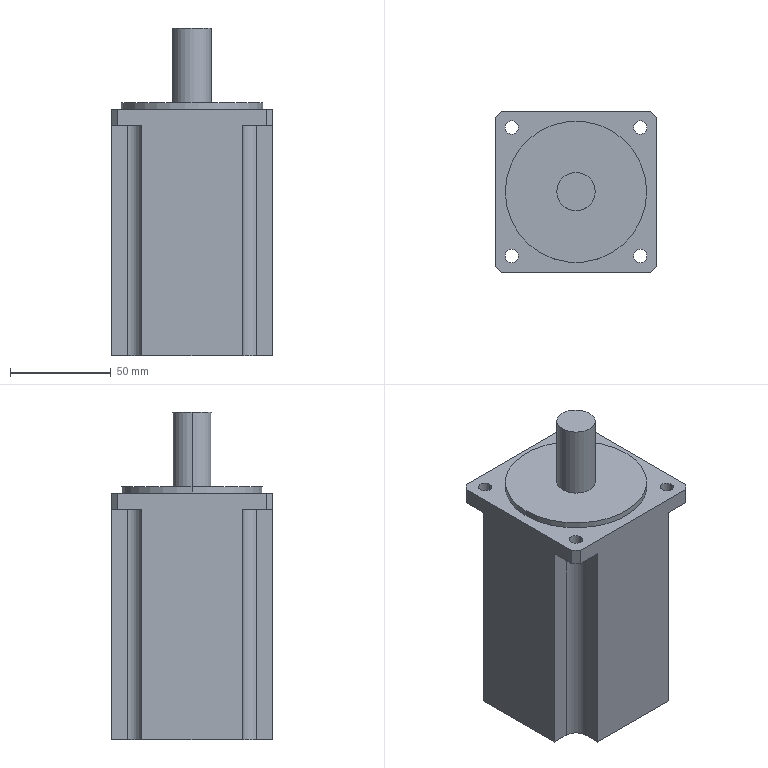Part | Creo | features CURVE 4, DATUM PLANE 3, PROTRUSION 3, CHAMFER 1, COORDINATE SYSTEM 1, CUT 1 | 1 solid | 40 faces | box 80 x 80 x 162.2 mm | volume 703450 mm3 | plane 24 | cylinder 16 | commonest cylinder face diameters 6.6 x8 13.834 x4 19 x2 70 x2
STEP:
#1=CARTESIAN_POINT('',(0.,0.,0.));
#2=DIRECTION('',(0.,0.,1.));
#3=DIRECTION('',(1.,0.,0.));
#4=AXIS2_PLACEMENT_3D('',#1,#2,#3);
#5=CARTESIAN_POINT('',(-24.903,40.,0.));
#6=VERTEX_POINT('',#5);
#7=CARTESIAN_POINT('',(-24.903,31.82,0.));
#8=VERTEX_POINT('',#7);
#9=CARTESIAN_POINT('',(-24.903,40.,0.));
#10=DIRECTION('',(0.,-1.,0.));
#11=VECTOR('',#10,8.18);
#12=LINE('',#9,#11);
#13=EDGE_CURVE('',#6,#8,#12,.T.);
#14=ORIENTED_EDGE('',*,*,#13,.T.);
#15=CARTESIAN_POINT('',(-31.82,24.903,0.));
#16=VERTEX_POINT('',#15);
#17=CARTESIAN_POINT('',(-31.82,31.82,0.));
#18=DIRECTION('',(0.,0.,-1.));
#19=DIRECTION('',(1.,0.,0.));
#20=AXIS2_PLACEMENT_3D('',#17,#18,#19);
#21=CIRCLE('',#20,6.917);
#22=EDGE_CURVE('',#8,#16,#21,.T.);
#23=ORIENTED_EDGE('',*,*,#22,.T.);
#24=CARTESIAN_POINT('',(-40.,24.903,0.));
#25=VERTEX_POINT('',#24);
#26=CARTESIAN_POINT('',(-40.,24.903,0.));
#27=DIRECTION('',(1.,0.,0.));
#28=VECTOR('',#27,8.18);
#29=LINE('',#26,#28);
#30=EDGE_CURVE('',#25,#16,#29,.T.);
#31=ORIENTED_EDGE('',*,*,#30,.F.);
#32=CARTESIAN_POINT('',(-40.,-24.903,0.));
#33=VERTEX_POINT('',#32);
#34=CARTESIAN_POINT('',(-40.,24.903,0.));
#35=DIRECTION('',(0.,-1.,0.));
#36=VECTOR('',#35,49.805);
#37=LINE('',#34,#36);
#38=EDGE_CURVE('',#25,#33,#37,.T.);
#39=ORIENTED_EDGE('',*,*,#38,.T.);
#40=CARTESIAN_POINT('',(-31.82,-24.903,0.));
#41=VERTEX_POINT('',#40);
#42=CARTESIAN_POINT('',(-40.,-24.903,0.));
#43=DIRECTION('',(1.,0.,0.));
#44=VECTOR('',#43,8.18);
#45=LINE('',#42,#44);
#46=EDGE_CURVE('',#33,#41,#45,.T.);
#47=ORIENTED_EDGE('',*,*,#46,.T.);
#48=CARTESIAN_POINT('',(-24.903,-31.82,0.));
#49=VERTEX_POINT('',#48);
#50=CARTESIAN_POINT('',(-31.82,-31.82,0.));
#51=DIRECTION('',(0.,0.,-1.));
#52=DIRECTION('',(0.,1.,0.));
#53=AXIS2_PLACEMENT_3D('',#50,#51,#52);
#54=CIRCLE('',#53,6.917);
#55=EDGE_CURVE('',#41,#49,#54,.T.);
#56=ORIENTED_EDGE('',*,*,#55,.T.);
#57=CARTESIAN_POINT('',(-24.903,-40.,0.));
#58=VERTEX_POINT('',#57);
#59=CARTESIAN_POINT('',(-24.903,-40.,0.));
#60=DIRECTION('',(0.,1.,0.));
#61=VECTOR('',#60,8.18);
#62=LINE('',#59,#61);
#63=EDGE_CURVE('',#58,#49,#62,.T.);
#64=ORIENTED_EDGE('',*,*,#63,.F.);
#65=CARTESIAN_POINT('',(24.903,-40.,0.));
#66=VERTEX_POINT('',#65);
#67=CARTESIAN_POINT('',(-24.903,-40.,0.));
#68=DIRECTION('',(1.,0.,0.));
#69=VECTOR('',#68,49.805);
#70=LINE('',#67,#69);
#71=EDGE_CURVE('',#58,#66,#70,.T.);
#72=ORIENTED_EDGE('',*,*,#71,.T.);
#73=CARTESIAN_POINT('',(24.903,-31.82,0.));
#74=VERTEX_POINT('',#73);
#75=CARTESIAN_POINT('',(24.903,-40.,0.));
#76=DIRECTION('',(0.,1.,0.));
#77=VECTOR('',#76,8.18);
#78=LINE('',#75,#77);
#79=EDGE_CURVE('',#66,#74,#78,.T.);
#80=ORIENTED_EDGE('',*,*,#79,.T.);
#81=CARTESIAN_POINT('',(31.82,-24.903,0.));
#82=VERTEX_POINT('',#81);
#83=CARTESIAN_POINT('',(31.82,-31.82,0.));
#84=DIRECTION('',(0.,0.,-1.));
#85=DIRECTION('',(-1.,0.,0.));
#86=AXIS2_PLACEMENT_3D('',#83,#84,#85);
#87=CIRCLE('',#86,6.917);
#88=EDGE_CURVE('',#74,#82,#87,.T.);
#89=ORIENTED_EDGE('',*,*,#88,.T.);
#90=CARTESIAN_POINT('',(40.,-24.903,0.));
#91=VERTEX_POINT('',#90);
#92=CARTESIAN_POINT('',(40.,-24.903,0.));
#93=DIRECTION('',(-1.,0.,0.));
#94=VECTOR('',#93,8.18);
#95=LINE('',#92,#94);
#96=EDGE_CURVE('',#91,#82,#95,.T.);
#97=ORIENTED_EDGE('',*,*,#96,.F.);
#98=CARTESIAN_POINT('',(40.,24.903,0.));
#99=VERTEX_POINT('',#98);
#100=CARTESIAN_POINT('',(40.,-24.903,0.));
#101=DIRECTION('',(0.,1.,0.));
#102=VECTOR('',#101,49.805);
#103=LINE('',#100,#102);
#104=EDGE_CURVE('',#91,#99,#103,.T.);
#105=ORIENTED_EDGE('',*,*,#104,.T.);
#106=CARTESIAN_POINT('',(31.82,24.903,0.));
#107=VERTEX_POINT('',#106);
#108=CARTESIAN_POINT('',(40.,24.903,0.));
#109=DIRECTION('',(-1.,0.,0.));
#110=VECTOR('',#109,8.18);
#111=LINE('',#108,#110);
#112=EDGE_CURVE('',#99,#107,#111,.T.);
#113=ORIENTED_EDGE('',*,*,#112,.T.);
#114=CARTESIAN_POINT('',(24.903,31.82,0.));
#115=VERTEX_POINT('',#114);
#116=CARTESIAN_POINT('',(31.82,31.82,0.));
#117=DIRECTION('',(0.,0.,-1.));
#118=DIRECTION('',(0.,-1.,0.));
#119=AXIS2_PLACEMENT_3D('',#116,#117,#118);
#120=CIRCLE('',#119,6.917);
#121=EDGE_CURVE('',#107,#115,#120,.T.);
#122=ORIENTED_EDGE('',*,*,#121,.T.);
#123=CARTESIAN_POINT('',(24.903,40.,0.));
#124=VERTEX_POINT('',#123);
#125=CARTESIAN_POINT('',(24.903,40.,0.));
#126=DIRECTION('',(0.,-1.,0.));
#127=VECTOR('',#126,8.18);
#128=LINE('',#125,#127);
#129=EDGE_CURVE('',#124,#115,#128,.T.);
#130=ORIENTED_EDGE('',*,*,#129,.F.);
#131=CARTESIAN_POINT('',(24.903,40.,0.));
#132=DIRECTION('',(-1.,0.,0.));
#133=VECTOR('',#132,49.805);
#134=LINE('',#131,#133);
#135=EDGE_CURVE('',#124,#6,#134,.T.);
#136=ORIENTED_EDGE('',*,*,#135,.T.);
#137=EDGE_LOOP('',(#14,#23,#31,#39,#47,#56,#64,#72,#80,#89,#97,#105,#113,#122,#130,#136));
#138=FACE_OUTER_BOUND('',#137,.F.);
#139=CARTESIAN_POINT('',(0.,0.,0.));
#140=DIRECTION('',(0.,0.,1.));
#141=DIRECTION('',(1.,0.,0.));
#142=AXIS2_PLACEMENT_3D('',#139,#140,#141);
#143=PLANE('',#142);
#144=ADVANCED_FACE('',(#138),#143,.F.);
#145=ORIENTED_EDGE('',*,*,#13,.F.);
#146=CARTESIAN_POINT('',(-24.903,40.,114.2));
#147=VERTEX_POINT('',#146);
#148=CARTESIAN_POINT('',(-24.903,40.,0.));
#149=DIRECTION('',(0.,0.,1.));
#150=VECTOR('',#149,114.2);
#151=LINE('',#148,#150);
#152=EDGE_CURVE('',#6,#147,#151,.T.);
#153=ORIENTED_EDGE('',*,*,#152,.T.);
#154=CARTESIAN_POINT('',(-24.903,31.82,114.2));
#155=VERTEX_POINT('',#154);
#156=CARTESIAN_POINT('',(-24.903,40.,114.2));
#157=DIRECTION('',(0.,-1.,0.));
#158=VECTOR('',#157,8.18);
#159=LINE('',#156,#158);
#160=EDGE_CURVE('',#147,#155,#159,.T.);
#161=ORIENTED_EDGE('',*,*,#160,.T.);
#162=CARTESIAN_POINT('',(-24.903,31.82,0.));
#163=DIRECTION('',(0.,0.,1.));
#164=VECTOR('',#163,114.2);
#165=LINE('',#162,#164);
#166=EDGE_CURVE('',#8,#155,#165,.T.);
#167=ORIENTED_EDGE('',*,*,#166,.F.);
#168=EDGE_LOOP('',(#145,#153,#161,#167));
#169=FACE_OUTER_BOUND('',#168,.F.);
#170=CARTESIAN_POINT('',(-24.903,40.,0.));
#171=DIRECTION('',(1.,0.,0.));
#172=DIRECTION('',(0.,-1.,0.));
#173=AXIS2_PLACEMENT_3D('',#170,#171,#172);
#174=PLANE('',#173);
#175=ADVANCED_FACE('',(#169),#174,.F.);
#176=CARTESIAN_POINT('',(-37.,40.,122.2));
#177=VERTEX_POINT('',#176);
#178=CARTESIAN_POINT('',(-37.,40.,114.2));
#179=VERTEX_POINT('',#178);
#180=CARTESIAN_POINT('',(-37.,40.,122.2));
#181=DIRECTION('',(0.,0.,-1.));
#182=VECTOR('',#181,8.);
#183=LINE('',#180,#182);
#184=EDGE_CURVE('',#177,#179,#183,.T.);
#185=ORIENTED_EDGE('',*,*,#184,.T.);
#186=CARTESIAN_POINT('',(-24.903,40.,114.2));
#187=DIRECTION('',(-1.,0.,0.));
#188=VECTOR('',#187,12.097);
#189=LINE('',#186,#188);
#190=EDGE_CURVE('',#147,#179,#189,.T.);
#191=ORIENTED_EDGE('',*,*,#190,.F.);
#192=ORIENTED_EDGE('',*,*,#152,.F.);
#193=ORIENTED_EDGE('',*,*,#135,.F.);
#194=CARTESIAN_POINT('',(24.903,40.,114.2));
#195=VERTEX_POINT('',#194);
#196=CARTESIAN_POINT('',(24.903,40.,0.));
#197=DIRECTION('',(0.,0.,1.));
#198=VECTOR('',#197,114.2);
#199=LINE('',#196,#198);
#200=EDGE_CURVE('',#124,#195,#199,.T.);
#201=ORIENTED_EDGE('',*,*,#200,.T.);
#202=CARTESIAN_POINT('',(37.,40.,114.2));
#203=VERTEX_POINT('',#202);
#204=CARTESIAN_POINT('',(37.,40.,114.2));
#205=DIRECTION('',(-1.,0.,0.));
#206=VECTOR('',#205,12.097);
#207=LINE('',#204,#206);
#208=EDGE_CURVE('',#203,#195,#207,.T.);
#209=ORIENTED_EDGE('',*,*,#208,.F.);
#210=CARTESIAN_POINT('',(37.,40.,122.2));
#211=VERTEX_POINT('',#210);
#212=CARTESIAN_POINT('',(37.,40.,122.2));
#213=DIRECTION('',(0.,0.,-1.));
#214=VECTOR('',#213,8.);
#215=LINE('',#212,#214);
#216=EDGE_CURVE('',#211,#203,#215,.T.);
#217=ORIENTED_EDGE('',*,*,#216,.F.);
#218=CARTESIAN_POINT('',(37.,40.,122.2));
#219=DIRECTION('',(-1.,0.,0.));
#220=VECTOR('',#219,74.);
#221=LINE('',#218,#220);
#222=EDGE_CURVE('',#211,#177,#221,.T.);
#223=ORIENTED_EDGE('',*,*,#222,.T.);
#224=EDGE_LOOP('',(#185,#191,#192,#193,#201,#209,#217,#223));
#225=FACE_OUTER_BOUND('',#224,.F.);
#226=CARTESIAN_POINT('',(40.,40.,0.));
#227=DIRECTION('',(0.,1.,0.));
#228=DIRECTION('',(-1.,0.,0.));
#229=AXIS2_PLACEMENT_3D('',#226,#227,#228);
#230=PLANE('',#229);
#231=ADVANCED_FACE('',(#225),#230,.T.);
#232=CARTESIAN_POINT('',(-40.,37.,114.2));
#233=VERTEX_POINT('',#232);
#234=CARTESIAN_POINT('',(-40.,37.,114.2));
#235=DIRECTION('',(0.7071,0.7071,0.));
#236=VECTOR('',#235,4.243);
#237=LINE('',#234,#236);
#238=EDGE_CURVE('',#233,#179,#237,.T.);
#239=ORIENTED_EDGE('',*,*,#238,.T.);
#240=ORIENTED_EDGE('',*,*,#184,.F.);
#241=CARTESIAN_POINT('',(-40.,37.,122.2));
#242=VERTEX_POINT('',#241);
#243=CARTESIAN_POINT('',(-37.,40.,122.2));
#244=DIRECTION('',(-0.7071,-0.7071,0.));
#245=VECTOR('',#244,4.243);
#246=LINE('',#243,#245);
#247=EDGE_CURVE('',#177,#242,#246,.T.);
#248=ORIENTED_EDGE('',*,*,#247,.T.);
#249=CARTESIAN_POINT('',(-40.,37.,122.2));
#250=DIRECTION('',(0.,0.,-1.));
#251=VECTOR('',#250,8.);
#252=LINE('',#249,#251);
#253=EDGE_CURVE('',#242,#233,#252,.T.);
#254=ORIENTED_EDGE('',*,*,#253,.T.);
#255=EDGE_LOOP('',(#239,#240,#248,#254));
#256=FACE_OUTER_BOUND('',#255,.F.);
#257=CARTESIAN_POINT('',(-38.5,38.5,118.2));
#258=DIRECTION('',(-0.7071,0.7071,0.));
#259=DIRECTION('',(0.7071,0.7071,0.));
#260=AXIS2_PLACEMENT_3D('',#257,#258,#259);
#261=PLANE('',#260);
#262=ADVANCED_FACE('',(#256),#261,.T.);
#263=ORIENTED_EDGE('',*,*,#238,.F.);
#264=CARTESIAN_POINT('',(-40.,24.903,114.2));
#265=VERTEX_POINT('',#264);
#266=CARTESIAN_POINT('',(-40.,37.,114.2));
#267=DIRECTION('',(0.,-1.,0.));
#268=VECTOR('',#267,12.097);
#269=LINE('',#266,#268);
#270=EDGE_CURVE('',#233,#265,#269,.T.);
#271=ORIENTED_EDGE('',*,*,#270,.T.);
#272=CARTESIAN_POINT('',(-31.82,24.903,114.2));
#273=VERTEX_POINT('',#272);
#274=CARTESIAN_POINT('',(-31.82,24.903,114.2));
#275=DIRECTION('',(-1.,0.,0.));
#276=VECTOR('',#275,8.18);
#277=LINE('',#274,#276);
#278=EDGE_CURVE('',#273,#265,#277,.T.);
#279=ORIENTED_EDGE('',*,*,#278,.F.);
#280=CARTESIAN_POINT('',(-31.82,31.82,114.2));
#281=DIRECTION('',(0.,0.,-1.));
#282=DIRECTION('',(1.,0.,0.));
#283=AXIS2_PLACEMENT_3D('',#280,#281,#282);
#284=CIRCLE('',#283,6.917);
#285=EDGE_CURVE('',#155,#273,#284,.T.);
#286=ORIENTED_EDGE('',*,*,#285,.F.);
#287=ORIENTED_EDGE('',*,*,#160,.F.);
#288=ORIENTED_EDGE('',*,*,#190,.T.);
#289=EDGE_LOOP('',(#263,#271,#279,#286,#287,#288));
#290=FACE_OUTER_BOUND('',#289,.F.);
#291=CARTESIAN_POINT('',(-35.12,31.82,114.2));
#292=VERTEX_POINT('',#291);
#293=CARTESIAN_POINT('',(-28.52,31.82,114.2));
#294=VERTEX_POINT('',#293);
#295=CARTESIAN_POINT('',(-31.82,31.82,114.2));
#296=DIRECTION('',(0.,0.,1.));
#297=DIRECTION('',(-1.,0.,0.));
#298=AXIS2_PLACEMENT_3D('',#295,#296,#297);
#299=CIRCLE('',#298,3.3);
#300=EDGE_CURVE('',#292,#294,#299,.T.);
#301=ORIENTED_EDGE('',*,*,#300,.F.);
#302=CARTESIAN_POINT('',(-31.82,31.82,114.2));
#303=DIRECTION('',(0.,0.,1.));
#304=DIRECTION('',(1.,0.,0.));
#305=AXIS2_PLACEMENT_3D('',#302,#303,#304);
#306=CIRCLE('',#305,3.3);
#307=EDGE_CURVE('',#294,#292,#306,.T.);
#308=ORIENTED_EDGE('',*,*,#307,.F.);
#309=EDGE_LOOP('',(#301,#308));
#310=FACE_BOUND('',#309,.F.);
#311=CARTESIAN_POINT('',(0.,0.,114.2));
#312=DIRECTION('',(0.,0.,-1.));
#313=DIRECTION('',(-1.,0.,0.));
#314=AXIS2_PLACEMENT_3D('',#311,#312,#313);
#315=PLANE('',#314);
#316=ADVANCED_FACE('',(#290,#310),#315,.T.);
#317=CARTESIAN_POINT('',(-37.,-40.,114.2));
#318=VERTEX_POINT('',#317);
#319=CARTESIAN_POINT('',(-40.,-37.,114.2));
#320=VERTEX_POINT('',#319);
#321=CARTESIAN_POINT('',(-37.,-40.,114.2));
#322=DIRECTION('',(-0.7071,0.7071,0.));
#323=VECTOR('',#322,4.243);
#324=LINE('',#321,#323);
#325=EDGE_CURVE('',#318,#320,#324,.T.);
#326=ORIENTED_EDGE('',*,*,#325,.F.);
#327=CARTESIAN_POINT('',(-24.903,-40.,114.2));
#328=VERTEX_POINT('',#327);
#329=CARTESIAN_POINT('',(-37.,-40.,114.2));
#330=DIRECTION('',(1.,0.,0.));
#331=VECTOR('',#330,12.097);
#332=LINE('',#329,#331);
#333=EDGE_CURVE('',#318,#328,#332,.T.);
#334=ORIENTED_EDGE('',*,*,#333,.T.);
#335=CARTESIAN_POINT('',(-24.903,-31.82,114.2));
#336=VERTEX_POINT('',#335);
#337=CARTESIAN_POINT('',(-24.903,-31.82,114.2));
#338=DIRECTION('',(0.,-1.,0.));
#339=VECTOR('',#338,8.18);
#340=LINE('',#337,#339);
#341=EDGE_CURVE('',#336,#328,#340,.T.);
#342=ORIENTED_EDGE('',*,*,#341,.F.);
#343=CARTESIAN_POINT('',(-31.82,-24.903,114.2));
#344=VERTEX_POINT('',#343);
#345=CARTESIAN_POINT('',(-31.82,-31.82,114.2));
#346=DIRECTION('',(0.,0.,-1.));
#347=DIRECTION('',(0.,1.,0.));
#348=AXIS2_PLACEMENT_3D('',#345,#346,#347);
#349=CIRCLE('',#348,6.917);
#350=EDGE_CURVE('',#344,#336,#349,.T.);
#351=ORIENTED_EDGE('',*,*,#350,.F.);
#352=CARTESIAN_POINT('',(-40.,-24.903,114.2));
#353=VERTEX_POINT('',#352);
#354=CARTESIAN_POINT('',(-40.,-24.903,114.2));
#355=DIRECTION('',(1.,0.,0.));
#356=VECTOR('',#355,8.18);
#357=LINE('',#354,#356);
#358=EDGE_CURVE('',#353,#344,#357,.T.);
#359=ORIENTED_EDGE('',*,*,#358,.F.);
#360=CARTESIAN_POINT('',(-40.,-24.903,114.2));
#361=DIRECTION('',(0.,-1.,0.));
#362=VECTOR('',#361,12.097);
#363=LINE('',#360,#362);
#364=EDGE_CURVE('',#353,#320,#363,.T.);
#365=ORIENTED_EDGE('',*,*,#364,.T.);
#366=EDGE_LOOP('',(#326,#334,#342,#351,#359,#365));
#367=FACE_OUTER_BOUND('',#366,.F.);
#368=CARTESIAN_POINT('',(-35.12,-31.82,114.2));
#369=VERTEX_POINT('',#368);
#370=CARTESIAN_POINT('',(-28.52,-31.82,114.2));
#371=VERTEX_POINT('',#370);
#372=CARTESIAN_POINT('',(-31.82,-31.82,114.2));
#373=DIRECTION('',(0.,0.,1.));
#374=DIRECTION('',(-1.,0.,0.));
#375=AXIS2_PLACEMENT_3D('',#372,#373,#374);
#376=CIRCLE('',#375,3.3);
#377=EDGE_CURVE('',#369,#371,#376,.T.);
#378=ORIENTED_EDGE('',*,*,#377,.F.);
#379=CARTESIAN_POINT('',(-31.82,-31.82,114.2));
#380=DIRECTION('',(0.,0.,1.));
#381=DIRECTION('',(1.,0.,0.));
#382=AXIS2_PLACEMENT_3D('',#379,#380,#381);
#383=CIRCLE('',#382,3.3);
#384=EDGE_CURVE('',#371,#369,#383,.T.);
#385=ORIENTED_EDGE('',*,*,#384,.F.);
#386=EDGE_LOOP('',(#378,#385));
#387=FACE_BOUND('',#386,.F.);
#388=CARTESIAN_POINT('',(0.,0.,114.2));
#389=DIRECTION('',(0.,0.,-1.));
#390=DIRECTION('',(-1.,0.,0.));
#391=AXIS2_PLACEMENT_3D('',#388,#389,#390);
#392=PLANE('',#391);
#393=ADVANCED_FACE('',(#367,#387),#392,.T.);
#394=CARTESIAN_POINT('',(40.,-37.,114.2));
#395=VERTEX_POINT('',#394);
#396=CARTESIAN_POINT('',(37.,-40.,114.2));
#397=VERTEX_POINT('',#396);
#398=CARTESIAN_POINT('',(40.,-37.,114.2));
#399=DIRECTION('',(-0.7071,-0.7071,0.));
#400=VECTOR('',#399,4.243);
#401=LINE('',#398,#400);
#402=EDGE_CURVE('',#395,#397,#401,.T.);
#403=ORIENTED_EDGE('',*,*,#402,.F.);
#404=CARTESIAN_POINT('',(40.,-24.903,114.2));
#405=VERTEX_POINT('',#404);
#406=CARTESIAN_POINT('',(40.,-37.,114.2));
#407=DIRECTION('',(0.,1.,0.));
#408=VECTOR('',#407,12.097);
#409=LINE('',#406,#408);
#410=EDGE_CURVE('',#395,#405,#409,.T.);
#411=ORIENTED_EDGE('',*,*,#410,.T.);
#412=CARTESIAN_POINT('',(31.82,-24.903,114.2));
#413=VERTEX_POINT('',#412);
#414=CARTESIAN_POINT('',(31.82,-24.903,114.2));
#415=DIRECTION('',(1.,0.,0.));
#416=VECTOR('',#415,8.18);
#417=LINE('',#414,#416);
#418=EDGE_CURVE('',#413,#405,#417,.T.);
#419=ORIENTED_EDGE('',*,*,#418,.F.);
#420=CARTESIAN_POINT('',(24.903,-31.82,114.2));
#421=VERTEX_POINT('',#420);
#422=CARTESIAN_POINT('',(31.82,-31.82,114.2));
#423=DIRECTION('',(0.,0.,-1.));
#424=DIRECTION('',(-1.,0.,0.));
#425=AXIS2_PLACEMENT_3D('',#422,#423,#424);
#426=CIRCLE('',#425,6.917);
#427=EDGE_CURVE('',#421,#413,#426,.T.);
#428=ORIENTED_EDGE('',*,*,#427,.F.);
#429=CARTESIAN_POINT('',(24.903,-40.,114.2));
#430=VERTEX_POINT('',#429);
#431=CARTESIAN_POINT('',(24.903,-40.,114.2));
#432=DIRECTION('',(0.,1.,0.));
#433=VECTOR('',#432,8.18);
#434=LINE('',#431,#433);
#435=EDGE_CURVE('',#430,#421,#434,.T.);
#436=ORIENTED_EDGE('',*,*,#435,.F.);
#437=CARTESIAN_POINT('',(24.903,-40.,114.2));
#438=DIRECTION('',(1.,0.,0.));
#439=VECTOR('',#438,12.097);
#440=LINE('',#437,#439);
#441=EDGE_CURVE('',#430,#397,#440,.T.);
#442=ORIENTED_EDGE('',*,*,#441,.T.);
#443=EDGE_LOOP('',(#403,#411,#419,#428,#436,#442));
#444=FACE_OUTER_BOUND('',#443,.F.);
#445=CARTESIAN_POINT('',(28.52,-31.82,114.2));
#446=VERTEX_POINT('',#445);
#447=CARTESIAN_POINT('',(35.12,-31.82,114.2));
#448=VERTEX_POINT('',#447);
#449=CARTESIAN_POINT('',(31.82,-31.82,114.2));
#450=DIRECTION('',(0.,0.,1.));
#451=DIRECTION('',(-1.,0.,0.));
#452=AXIS2_PLACEMENT_3D('',#449,#450,#451);
#453=CIRCLE('',#452,3.3);
#454=EDGE_CURVE('',#446,#448,#453,.T.);
#455=ORIENTED_EDGE('',*,*,#454,.F.);
#456=CARTESIAN_POINT('',(31.82,-31.82,114.2));
#457=DIRECTION('',(0.,0.,1.));
#458=DIRECTION('',(1.,0.,0.));
#459=AXIS2_PLACEMENT_3D('',#456,#457,#458);
#460=CIRCLE('',#459,3.3);
#461=EDGE_CURVE('',#448,#446,#460,.T.);
#462=ORIENTED_EDGE('',*,*,#461,.F.);
#463=EDGE_LOOP('',(#455,#462));
#464=FACE_BOUND('',#463,.F.);
#465=CARTESIAN_POINT('',(0.,0.,114.2));
#466=DIRECTION('',(0.,0.,-1.));
#467=DIRECTION('',(-1.,0.,0.));
#468=AXIS2_PLACEMENT_3D('',#465,#466,#467);
#469=PLANE('',#468);
#470=ADVANCED_FACE('',(#444,#464),#469,.T.);
#471=CARTESIAN_POINT('',(40.,37.,114.2));
#472=VERTEX_POINT('',#471);
#473=CARTESIAN_POINT('',(37.,40.,114.2));
#474=DIRECTION('',(0.7071,-0.7071,0.));
#475=VECTOR('',#474,4.243);
#476=LINE('',#473,#475);
#477=EDGE_CURVE('',#203,#472,#476,.T.);
#478=ORIENTED_EDGE('',*,*,#477,.F.);
#479=ORIENTED_EDGE('',*,*,#208,.T.);
#480=CARTESIAN_POINT('',(24.903,31.82,114.2));
#481=VERTEX_POINT('',#480);
#482=CARTESIAN_POINT('',(24.903,31.82,114.2));
#483=DIRECTION('',(0.,1.,0.));
#484=VECTOR('',#483,8.18);
#485=LINE('',#482,#484);
#486=EDGE_CURVE('',#481,#195,#485,.T.);
#487=ORIENTED_EDGE('',*,*,#486,.F.);
#488=CARTESIAN_POINT('',(31.82,24.903,114.2));
#489=VERTEX_POINT('',#488);
#490=CARTESIAN_POINT('',(31.82,31.82,114.2));
#491=DIRECTION('',(0.,0.,-1.));
#492=DIRECTION('',(0.,-1.,0.));
#493=AXIS2_PLACEMENT_3D('',#490,#491,#492);
#494=CIRCLE('',#493,6.917);
#495=EDGE_CURVE('',#489,#481,#494,.T.);
#496=ORIENTED_EDGE('',*,*,#495,.F.);
#497=CARTESIAN_POINT('',(40.,24.903,114.2));
#498=VERTEX_POINT('',#497);
#499=CARTESIAN_POINT('',(40.,24.903,114.2));
#500=DIRECTION('',(-1.,0.,0.));
#501=VECTOR('',#500,8.18);
#502=LINE('',#499,#501);
#503=EDGE_CURVE('',#498,#489,#502,.T.);
#504=ORIENTED_EDGE('',*,*,#503,.F.);
#505=CARTESIAN_POINT('',(40.,24.903,114.2));
#506=DIRECTION('',(0.,1.,0.));
#507=VECTOR('',#506,12.097);
#508=LINE('',#505,#507);
#509=EDGE_CURVE('',#498,#472,#508,.T.);
#510=ORIENTED_EDGE('',*,*,#509,.T.);
#511=EDGE_LOOP('',(#478,#479,#487,#496,#504,#510));
#512=FACE_OUTER_BOUND('',#511,.F.);
#513=CARTESIAN_POINT('',(28.52,31.82,114.2));
#514=VERTEX_POINT('',#513);
#515=CARTESIAN_POINT('',(35.12,31.82,114.2));
#516=VERTEX_POINT('',#515);
#517=CARTESIAN_POINT('',(31.82,31.82,114.2));
#518=DIRECTION('',(0.,0.,1.));
#519=DIRECTION('',(-1.,0.,0.));
#520=AXIS2_PLACEMENT_3D('',#517,#518,#519);
#521=CIRCLE('',#520,3.3);
#522=EDGE_CURVE('',#514,#516,#521,.T.);
#523=ORIENTED_EDGE('',*,*,#522,.F.);
#524=CARTESIAN_POINT('',(31.82,31.82,114.2));
#525=DIRECTION('',(0.,0.,1.));
#526=DIRECTION('',(1.,0.,0.));
#527=AXIS2_PLACEMENT_3D('',#524,#525,#526);
#528=CIRCLE('',#527,3.3);
#529=EDGE_CURVE('',#516,#514,#528,.T.);
#530=ORIENTED_EDGE('',*,*,#529,.F.);
#531=EDGE_LOOP('',(#523,#530));
#532=FACE_BOUND('',#531,.F.);
#533=CARTESIAN_POINT('',(0.,0.,114.2));
#534=DIRECTION('',(0.,0.,-1.));
#535=DIRECTION('',(-1.,0.,0.));
#536=AXIS2_PLACEMENT_3D('',#533,#534,#535);
#537=PLANE('',#536);
#538=ADVANCED_FACE('',(#512,#532),#537,.T.);
#539=ORIENTED_EDGE('',*,*,#454,.T.);
#540=CARTESIAN_POINT('',(35.12,-31.82,122.2));
#541=VERTEX_POINT('',#540);
#542=CARTESIAN_POINT('',(35.12,-31.82,114.2));
#543=DIRECTION('',(0.,0.,1.));
#544=VECTOR('',#543,8.);
#545=LINE('',#542,#544);
#546=EDGE_CURVE('',#448,#541,#545,.T.);
#547=ORIENTED_EDGE('',*,*,#546,.T.);
#548=CARTESIAN_POINT('',(28.52,-31.82,122.2));
#549=VERTEX_POINT('',#548);
#550=CARTESIAN_POINT('',(31.82,-31.82,122.2));
#551=DIRECTION('',(0.,0.,-1.));
#552=DIRECTION('',(1.,0.,0.));
#553=AXIS2_PLACEMENT_3D('',#550,#551,#552);
#554=CIRCLE('',#553,3.3);
#555=EDGE_CURVE('',#541,#549,#554,.T.);
#556=ORIENTED_EDGE('',*,*,#555,.T.);
#557=CARTESIAN_POINT('',(28.52,-31.82,114.2));
#558=DIRECTION('',(0.,0.,1.));
#559=VECTOR('',#558,8.);
#560=LINE('',#557,#559);
#561=EDGE_CURVE('',#446,#549,#560,.T.);
#562=ORIENTED_EDGE('',*,*,#561,.F.);
#563=EDGE_LOOP('',(#539,#547,#556,#562));
#564=FACE_OUTER_BOUND('',#563,.F.);
#565=CARTESIAN_POINT('',(31.82,-31.82,0.));
#566=DIRECTION('',(0.,0.,1.));
#567=DIRECTION('',(1.,0.,0.));
#568=AXIS2_PLACEMENT_3D('',#565,#566,#567);
#569=CYLINDRICAL_SURFACE('',#568,3.3);
#570=ADVANCED_FACE('',(#564),#569,.F.);
#571=ORIENTED_EDGE('',*,*,#461,.T.);
#572=ORIENTED_EDGE('',*,*,#561,.T.);
#573=CARTESIAN_POINT('',(31.82,-31.82,122.2));
#574=DIRECTION('',(0.,0.,-1.));
#575=DIRECTION('',(-1.,0.,0.));
#576=AXIS2_PLACEMENT_3D('',#573,#574,#575);
#577=CIRCLE('',#576,3.3);
#578=EDGE_CURVE('',#549,#541,#577,.T.);
#579=ORIENTED_EDGE('',*,*,#578,.T.);
#580=ORIENTED_EDGE('',*,*,#546,.F.);
#581=EDGE_LOOP('',(#571,#572,#579,#580));
#582=FACE_OUTER_BOUND('',#581,.F.);
#583=CARTESIAN_POINT('',(31.82,-31.82,0.));
#584=DIRECTION('',(0.,0.,1.));
#585=DIRECTION('',(1.,0.,0.));
#586=AXIS2_PLACEMENT_3D('',#583,#584,#585);
#587=CYLINDRICAL_SURFACE('',#586,3.3);
#588=ADVANCED_FACE('',(#582),#587,.F.);
#589=ORIENTED_EDGE('',*,*,#247,.F.);
#590=ORIENTED_EDGE('',*,*,#222,.F.);
#591=CARTESIAN_POINT('',(40.,37.,122.2));
#592=VERTEX_POINT('',#591);
#593=CARTESIAN_POINT('',(40.,37.,122.2));
#594=DIRECTION('',(-0.7071,0.7071,0.));
#595=VECTOR('',#594,4.243);
#596=LINE('',#593,#595);
#597=EDGE_CURVE('',#592,#211,#596,.T.);
#598=ORIENTED_EDGE('',*,*,#597,.F.);
#599=CARTESIAN_POINT('',(40.,-37.,122.2));
#600=VERTEX_POINT('',#599);
#601=CARTESIAN_POINT('',(40.,-37.,122.2));
#602=DIRECTION('',(0.,1.,0.));
#603=VECTOR('',#602,74.);
#604=LINE('',#601,#603);
#605=EDGE_CURVE('',#600,#592,#604,.T.);
#606=ORIENTED_EDGE('',*,*,#605,.F.);
#607=CARTESIAN_POINT('',(37.,-40.,122.2));
#608=VERTEX_POINT('',#607);
#609=CARTESIAN_POINT('',(37.,-40.,122.2));
#610=DIRECTION('',(0.7071,0.7071,0.));
#611=VECTOR('',#610,4.243);
#612=LINE('',#609,#611);
#613=EDGE_CURVE('',#608,#600,#612,.T.);
#614=ORIENTED_EDGE('',*,*,#613,.F.);
#615=CARTESIAN_POINT('',(-37.,-40.,122.2));
#616=VERTEX_POINT('',#615);
#617=CARTESIAN_POINT('',(-37.,-40.,122.2));
#618=DIRECTION('',(1.,0.,0.));
#619=VECTOR('',#618,74.);
#620=LINE('',#617,#619);
#621=EDGE_CURVE('',#616,#608,#620,.T.);
#622=ORIENTED_EDGE('',*,*,#621,.F.);
#623=CARTESIAN_POINT('',(-40.,-37.,122.2));
#624=VERTEX_POINT('',#623);
#625=CARTESIAN_POINT('',(-40.,-37.,122.2));
#626=DIRECTION('',(0.7071,-0.7071,0.));
#627=VECTOR('',#626,4.243);
#628=LINE('',#625,#627);
#629=EDGE_CURVE('',#624,#616,#628,.T.);
#630=ORIENTED_EDGE('',*,*,#629,.F.);
#631=CARTESIAN_POINT('',(-40.,37.,122.2));
#632=DIRECTION('',(0.,-1.,0.));
#633=VECTOR('',#632,74.);
#634=LINE('',#631,#633);
#635=EDGE_CURVE('',#242,#624,#634,.T.);
#636=ORIENTED_EDGE('',*,*,#635,.F.);
#637=EDGE_LOOP('',(#589,#590,#598,#606,#614,#622,#630,#636));
#638=FACE_OUTER_BOUND('',#637,.F.);
#639=CARTESIAN_POINT('',(-28.52,31.82,122.2));
#640=VERTEX_POINT('',#639);
#641=CARTESIAN_POINT('',(-35.12,31.82,122.2));
#642=VERTEX_POINT('',#641);
#643=CARTESIAN_POINT('',(-31.82,31.82,122.2));
#644=DIRECTION('',(0.,0.,-1.));
#645=DIRECTION('',(1.,0.,0.));
#646=AXIS2_PLACEMENT_3D('',#643,#644,#645);
#647=CIRCLE('',#646,3.3);
#648=EDGE_CURVE('',#640,#642,#647,.T.);
#649=ORIENTED_EDGE('',*,*,#648,.F.);
#650=CARTESIAN_POINT('',(-31.82,31.82,122.2));
#651=DIRECTION('',(0.,0.,-1.));
#652=DIRECTION('',(-1.,0.,0.));
#653=AXIS2_PLACEMENT_3D('',#650,#651,#652);
#654=CIRCLE('',#653,3.3);
#655=EDGE_CURVE('',#642,#640,#654,.T.);
#656=ORIENTED_EDGE('',*,*,#655,.F.);
#657=EDGE_LOOP('',(#649,#656));
#658=FACE_BOUND('',#657,.F.);
#659=CARTESIAN_POINT('',(-28.52,-31.82,122.2));
#660=VERTEX_POINT('',#659);
#661=CARTESIAN_POINT('',(-35.12,-31.82,122.2));
#662=VERTEX_POINT('',#661);
#663=CARTESIAN_POINT('',(-31.82,-31.82,122.2));
#664=DIRECTION('',(0.,0.,-1.));
#665=DIRECTION('',(1.,0.,0.));
#666=AXIS2_PLACEMENT_3D('',#663,#664,#665);
#667=CIRCLE('',#666,3.3);
#668=EDGE_CURVE('',#660,#662,#667,.T.);
#669=ORIENTED_EDGE('',*,*,#668,.F.);
#670=CARTESIAN_POINT('',(-31.82,-31.82,122.2));
#671=DIRECTION('',(0.,0.,-1.));
#672=DIRECTION('',(-1.,0.,0.));
#673=AXIS2_PLACEMENT_3D('',#670,#671,#672);
#674=CIRCLE('',#673,3.3);
#675=EDGE_CURVE('',#662,#660,#674,.T.);
#676=ORIENTED_EDGE('',*,*,#675,.F.);
#677=EDGE_LOOP('',(#669,#676));
#678=FACE_BOUND('',#677,.F.);
#679=ORIENTED_EDGE('',*,*,#555,.F.);
#680=ORIENTED_EDGE('',*,*,#578,.F.);
#681=EDGE_LOOP('',(#679,#680));
#682=FACE_BOUND('',#681,.F.);
#683=CARTESIAN_POINT('',(35.,0.,122.2));
#684=VERTEX_POINT('',#683);
#685=CARTESIAN_POINT('',(-35.,0.,122.2));
#686=VERTEX_POINT('',#685);
#687=CARTESIAN_POINT('',(0.,0.,122.2));
#688=DIRECTION('',(0.,0.,1.));
#689=DIRECTION('',(1.,0.,0.));
#690=AXIS2_PLACEMENT_3D('',#687,#688,#689);
#691=CIRCLE('',#690,35.);
#692=EDGE_CURVE('',#684,#686,#691,.T.);
#693=ORIENTED_EDGE('',*,*,#692,.T.);
#694=CARTESIAN_POINT('',(0.,0.,122.2));
#695=DIRECTION('',(0.,0.,1.));
#696=DIRECTION('',(-1.,0.,0.));
#697=AXIS2_PLACEMENT_3D('',#694,#695,#696);
#698=CIRCLE('',#697,35.);
#699=EDGE_CURVE('',#686,#684,#698,.T.);
#700=ORIENTED_EDGE('',*,*,#699,.T.);
#701=EDGE_LOOP('',(#693,#700));
#702=FACE_BOUND('',#701,.F.);
#703=CARTESIAN_POINT('',(35.12,31.82,122.2));
#704=VERTEX_POINT('',#703);
#705=CARTESIAN_POINT('',(28.52,31.82,122.2));
#706=VERTEX_POINT('',#705);
#707=CARTESIAN_POINT('',(31.82,31.82,122.2));
#708=DIRECTION('',(0.,0.,-1.));
#709=DIRECTION('',(1.,0.,0.));
#710=AXIS2_PLACEMENT_3D('',#707,#708,#709);
#711=CIRCLE('',#710,3.3);
#712=EDGE_CURVE('',#704,#706,#711,.T.);
#713=ORIENTED_EDGE('',*,*,#712,.F.);
#714=CARTESIAN_POINT('',(31.82,31.82,122.2));
#715=DIRECTION('',(0.,0.,-1.));
#716=DIRECTION('',(-1.,0.,0.));
#717=AXIS2_PLACEMENT_3D('',#714,#715,#716);
#718=CIRCLE('',#717,3.3);
#719=EDGE_CURVE('',#706,#704,#718,.T.);
#720=ORIENTED_EDGE('',*,*,#719,.F.);
#721=EDGE_LOOP('',(#713,#720));
#722=FACE_BOUND('',#721,.F.);
#723=CARTESIAN_POINT('',(0.,0.,122.2));
#724=DIRECTION('',(0.,0.,1.));
#725=DIRECTION('',(1.,0.,0.));
#726=AXIS2_PLACEMENT_3D('',#723,#724,#725);
#727=PLANE('',#726);
#728=ADVANCED_FACE('',(#638,#658,#678,#682,#702,#722),#727,.T.);
#729=ORIENTED_EDGE('',*,*,#522,.T.);
#730=CARTESIAN_POINT('',(35.12,31.82,114.2));
#731=DIRECTION('',(0.,0.,1.));
#732=VECTOR('',#731,8.);
#733=LINE('',#730,#732);
#734=EDGE_CURVE('',#516,#704,#733,.T.);
#735=ORIENTED_EDGE('',*,*,#734,.T.);
#736=ORIENTED_EDGE('',*,*,#712,.T.);
#737=CARTESIAN_POINT('',(28.52,31.82,114.2));
#738=DIRECTION('',(0.,0.,1.));
#739=VECTOR('',#738,8.);
#740=LINE('',#737,#739);
#741=EDGE_CURVE('',#514,#706,#740,.T.);
#742=ORIENTED_EDGE('',*,*,#741,.F.);
#743=EDGE_LOOP('',(#729,#735,#736,#742));
#744=FACE_OUTER_BOUND('',#743,.F.);
#745=CARTESIAN_POINT('',(31.82,31.82,0.));
#746=DIRECTION('',(0.,0.,1.));
#747=DIRECTION('',(1.,0.,0.));
#748=AXIS2_PLACEMENT_3D('',#745,#746,#747);
#749=CYLINDRICAL_SURFACE('',#748,3.3);
#750=ADVANCED_FACE('',(#744),#749,.F.);
#751=ORIENTED_EDGE('',*,*,#529,.T.);
#752=ORIENTED_EDGE('',*,*,#741,.T.);
#753=ORIENTED_EDGE('',*,*,#719,.T.);
#754=ORIENTED_EDGE('',*,*,#734,.F.);
#755=EDGE_LOOP('',(#751,#752,#753,#754));
#756=FACE_OUTER_BOUND('',#755,.F.);
#757=CARTESIAN_POINT('',(31.82,31.82,0.));
#758=DIRECTION('',(0.,0.,1.));
#759=DIRECTION('',(1.,0.,0.));
#760=AXIS2_PLACEMENT_3D('',#757,#758,#759);
#761=CYLINDRICAL_SURFACE('',#760,3.3);
#762=ADVANCED_FACE('',(#756),#761,.F.);
#763=ORIENTED_EDGE('',*,*,#300,.T.);
#764=CARTESIAN_POINT('',(-28.52,31.82,114.2));
#765=DIRECTION('',(0.,0.,1.));
#766=VECTOR('',#765,8.);
#767=LINE('',#764,#766);
#768=EDGE_CURVE('',#294,#640,#767,.T.);
#769=ORIENTED_EDGE('',*,*,#768,.T.);
#770=ORIENTED_EDGE('',*,*,#648,.T.);
#771=CARTESIAN_POINT('',(-35.12,31.82,114.2));
#772=DIRECTION('',(0.,0.,1.));
#773=VECTOR('',#772,8.);
#774=LINE('',#771,#773);
#775=EDGE_CURVE('',#292,#642,#774,.T.);
#776=ORIENTED_EDGE('',*,*,#775,.F.);
#777=EDGE_LOOP('',(#763,#769,#770,#776));
#778=FACE_OUTER_BOUND('',#777,.F.);
#779=CARTESIAN_POINT('',(-31.82,31.82,0.));
#780=DIRECTION('',(0.,0.,1.));
#781=DIRECTION('',(1.,0.,0.));
#782=AXIS2_PLACEMENT_3D('',#779,#780,#781);
#783=CYLINDRICAL_SURFACE('',#782,3.3);
#784=ADVANCED_FACE('',(#778),#783,.F.);
#785=ORIENTED_EDGE('',*,*,#307,.T.);
#786=ORIENTED_EDGE('',*,*,#775,.T.);
#787=ORIENTED_EDGE('',*,*,#655,.T.);
#788=ORIENTED_EDGE('',*,*,#768,.F.);
#789=EDGE_LOOP('',(#785,#786,#787,#788));
#790=FACE_OUTER_BOUND('',#789,.F.);
#791=CARTESIAN_POINT('',(-31.82,31.82,0.));
#792=DIRECTION('',(0.,0.,1.));
#793=DIRECTION('',(1.,0.,0.));
#794=AXIS2_PLACEMENT_3D('',#791,#792,#793);
#795=CYLINDRICAL_SURFACE('',#794,3.3);
#796=ADVANCED_FACE('',(#790),#795,.F.);
#797=ORIENTED_EDGE('',*,*,#377,.T.);
#798=CARTESIAN_POINT('',(-28.52,-31.82,114.2));
#799=DIRECTION('',(0.,0.,1.));
#800=VECTOR('',#799,8.);
#801=LINE('',#798,#800);
#802=EDGE_CURVE('',#371,#660,#801,.T.);
#803=ORIENTED_EDGE('',*,*,#802,.T.);
#804=ORIENTED_EDGE('',*,*,#668,.T.);
#805=CARTESIAN_POINT('',(-35.12,-31.82,114.2));
#806=DIRECTION('',(0.,0.,1.));
#807=VECTOR('',#806,8.);
#808=LINE('',#805,#807);
#809=EDGE_CURVE('',#369,#662,#808,.T.);
#810=ORIENTED_EDGE('',*,*,#809,.F.);
#811=EDGE_LOOP('',(#797,#803,#804,#810));
#812=FACE_OUTER_BOUND('',#811,.F.);
#813=CARTESIAN_POINT('',(-31.82,-31.82,0.));
#814=DIRECTION('',(0.,0.,1.));
#815=DIRECTION('',(1.,0.,0.));
#816=AXIS2_PLACEMENT_3D('',#813,#814,#815);
#817=CYLINDRICAL_SURFACE('',#816,3.3);
#818=ADVANCED_FACE('',(#812),#817,.F.);
#819=ORIENTED_EDGE('',*,*,#384,.T.);
#820=ORIENTED_EDGE('',*,*,#809,.T.);
#821=ORIENTED_EDGE('',*,*,#675,.T.);
#822=ORIENTED_EDGE('',*,*,#802,.F.);
#823=EDGE_LOOP('',(#819,#820,#821,#822));
#824=FACE_OUTER_BOUND('',#823,.F.);
#825=CARTESIAN_POINT('',(-31.82,-31.82,0.));
#826=DIRECTION('',(0.,0.,1.));
#827=DIRECTION('',(1.,0.,0.));
#828=AXIS2_PLACEMENT_3D('',#825,#826,#827);
#829=CYLINDRICAL_SURFACE('',#828,3.3);
#830=ADVANCED_FACE('',(#824),#829,.F.);
#831=ORIENTED_EDGE('',*,*,#692,.F.);
#832=CARTESIAN_POINT('',(35.,0.,125.2));
#833=VERTEX_POINT('',#832);
#834=CARTESIAN_POINT('',(35.,0.,122.2));
#835=DIRECTION('',(0.,0.,1.));
#836=VECTOR('',#835,3.);
#837=LINE('',#834,#836);
#838=EDGE_CURVE('',#684,#833,#837,.T.);
#839=ORIENTED_EDGE('',*,*,#838,.T.);
#840=CARTESIAN_POINT('',(-35.,0.,125.2));
#841=VERTEX_POINT('',#840);
#842=CARTESIAN_POINT('',(0.,0.,125.2));
#843=DIRECTION('',(0.,0.,1.));
#844=DIRECTION('',(1.,0.,0.));
#845=AXIS2_PLACEMENT_3D('',#842,#843,#844);
#846=CIRCLE('',#845,35.);
#847=EDGE_CURVE('',#833,#841,#846,.T.);
#848=ORIENTED_EDGE('',*,*,#847,.T.);
#849=CARTESIAN_POINT('',(-35.,0.,122.2));
#850=DIRECTION('',(0.,0.,1.));
#851=VECTOR('',#850,3.);
#852=LINE('',#849,#851);
#853=EDGE_CURVE('',#686,#841,#852,.T.);
#854=ORIENTED_EDGE('',*,*,#853,.F.);
#855=EDGE_LOOP('',(#831,#839,#848,#854));
#856=FACE_OUTER_BOUND('',#855,.F.);
#857=CARTESIAN_POINT('',(0.,0.,122.2));
#858=DIRECTION('',(0.,0.,1.));
#859=DIRECTION('',(1.,0.,0.));
#860=AXIS2_PLACEMENT_3D('',#857,#858,#859);
#861=CYLINDRICAL_SURFACE('',#860,35.);
#862=ADVANCED_FACE('',(#856),#861,.T.);
#863=ORIENTED_EDGE('',*,*,#699,.F.);
#864=ORIENTED_EDGE('',*,*,#853,.T.);
#865=CARTESIAN_POINT('',(0.,0.,125.2));
#866=DIRECTION('',(0.,0.,1.));
#867=DIRECTION('',(-1.,0.,0.));
#868=AXIS2_PLACEMENT_3D('',#865,#866,#867);
#869=CIRCLE('',#868,35.);
#870=EDGE_CURVE('',#841,#833,#869,.T.);
#871=ORIENTED_EDGE('',*,*,#870,.T.);
#872=ORIENTED_EDGE('',*,*,#838,.F.);
#873=EDGE_LOOP('',(#863,#864,#871,#872));
#874=FACE_OUTER_BOUND('',#873,.F.);
#875=CARTESIAN_POINT('',(0.,0.,122.2));
#876=DIRECTION('',(0.,0.,1.));
#877=DIRECTION('',(1.,0.,0.));
#878=AXIS2_PLACEMENT_3D('',#875,#876,#877);
#879=CYLINDRICAL_SURFACE('',#878,35.);
#880=ADVANCED_FACE('',(#874),#879,.T.);
#881=ORIENTED_EDGE('',*,*,#847,.F.);
#882=ORIENTED_EDGE('',*,*,#870,.F.);
#883=EDGE_LOOP('',(#881,#882));
#884=FACE_OUTER_BOUND('',#883,.F.);
#885=CARTESIAN_POINT('',(9.5,0.,125.2));
#886=VERTEX_POINT('',#885);
#887=CARTESIAN_POINT('',(-9.5,0.,125.2));
#888=VERTEX_POINT('',#887);
#889=CARTESIAN_POINT('',(0.,0.,125.2));
#890=DIRECTION('',(0.,0.,1.));
#891=DIRECTION('',(1.,0.,0.));
#892=AXIS2_PLACEMENT_3D('',#889,#890,#891);
#893=CIRCLE('',#892,9.5);
#894=EDGE_CURVE('',#886,#888,#893,.T.);
#895=ORIENTED_EDGE('',*,*,#894,.T.);
#896=CARTESIAN_POINT('',(0.,0.,125.2));
#897=DIRECTION('',(0.,0.,1.));
#898=DIRECTION('',(-1.,0.,0.));
#899=AXIS2_PLACEMENT_3D('',#896,#897,#898);
#900=CIRCLE('',#899,9.5);
#901=EDGE_CURVE('',#888,#886,#900,.T.);
#902=ORIENTED_EDGE('',*,*,#901,.T.);
#903=EDGE_LOOP('',(#895,#902));
#904=FACE_BOUND('',#903,.F.);
#905=CARTESIAN_POINT('',(0.,0.,125.2));
#906=DIRECTION('',(0.,0.,1.));
#907=DIRECTION('',(1.,0.,0.));
#908=AXIS2_PLACEMENT_3D('',#905,#906,#907);
#909=PLANE('',#908);
#910=ADVANCED_FACE('',(#884,#904),#909,.T.);
#911=ORIENTED_EDGE('',*,*,#894,.F.);
#912=CARTESIAN_POINT('',(9.5,0.,162.2));
#913=VERTEX_POINT('',#912);
#914=CARTESIAN_POINT('',(9.5,0.,125.2));
#915=DIRECTION('',(0.,0.,1.));
#916=VECTOR('',#915,37.);
#917=LINE('',#914,#916);
#918=EDGE_CURVE('',#886,#913,#917,.T.);
#919=ORIENTED_EDGE('',*,*,#918,.T.);
#920=CARTESIAN_POINT('',(-9.5,0.,162.2));
#921=VERTEX_POINT('',#920);
#922=CARTESIAN_POINT('',(0.,0.,162.2));
#923=DIRECTION('',(0.,0.,1.));
#924=DIRECTION('',(1.,0.,0.));
#925=AXIS2_PLACEMENT_3D('',#922,#923,#924);
#926=CIRCLE('',#925,9.5);
#927=EDGE_CURVE('',#913,#921,#926,.T.);
#928=ORIENTED_EDGE('',*,*,#927,.T.);
#929=CARTESIAN_POINT('',(-9.5,0.,125.2));
#930=DIRECTION('',(0.,0.,1.));
#931=VECTOR('',#930,37.);
#932=LINE('',#929,#931);
#933=EDGE_CURVE('',#888,#921,#932,.T.);
#934=ORIENTED_EDGE('',*,*,#933,.F.);
#935=EDGE_LOOP('',(#911,#919,#928,#934));
#936=FACE_OUTER_BOUND('',#935,.F.);
#937=CARTESIAN_POINT('',(0.,0.,125.2));
#938=DIRECTION('',(0.,0.,1.));
#939=DIRECTION('',(1.,0.,0.));
#940=AXIS2_PLACEMENT_3D('',#937,#938,#939);
#941=CYLINDRICAL_SURFACE('',#940,9.5);
#942=ADVANCED_FACE('',(#936),#941,.T.);
#943=ORIENTED_EDGE('',*,*,#901,.F.);
#944=ORIENTED_EDGE('',*,*,#933,.T.);
#945=CARTESIAN_POINT('',(0.,0.,162.2));
#946=DIRECTION('',(0.,0.,1.));
#947=DIRECTION('',(-1.,0.,0.));
#948=AXIS2_PLACEMENT_3D('',#945,#946,#947);
#949=CIRCLE('',#948,9.5);
#950=EDGE_CURVE('',#921,#913,#949,.T.);
#951=ORIENTED_EDGE('',*,*,#950,.T.);
#952=ORIENTED_EDGE('',*,*,#918,.F.);
#953=EDGE_LOOP('',(#943,#944,#951,#952));
#954=FACE_OUTER_BOUND('',#953,.F.);
#955=CARTESIAN_POINT('',(0.,0.,125.2));
#956=DIRECTION('',(0.,0.,1.));
#957=DIRECTION('',(1.,0.,0.));
#958=AXIS2_PLACEMENT_3D('',#955,#956,#957);
#959=CYLINDRICAL_SURFACE('',#958,9.5);
#960=ADVANCED_FACE('',(#954),#959,.T.);
#961=ORIENTED_EDGE('',*,*,#927,.F.);
#962=ORIENTED_EDGE('',*,*,#950,.F.);
#963=EDGE_LOOP('',(#961,#962));
#964=FACE_OUTER_BOUND('',#963,.F.);
#965=CARTESIAN_POINT('',(0.,0.,162.2));
#966=DIRECTION('',(0.,0.,1.));
#967=DIRECTION('',(1.,0.,0.));
#968=AXIS2_PLACEMENT_3D('',#965,#966,#967);
#969=PLANE('',#968);
#970=ADVANCED_FACE('',(#964),#969,.T.);
#971=ORIENTED_EDGE('',*,*,#477,.T.);
#972=CARTESIAN_POINT('',(40.,37.,122.2));
#973=DIRECTION('',(0.,0.,-1.));
#974=VECTOR('',#973,8.);
#975=LINE('',#972,#974);
#976=EDGE_CURVE('',#592,#472,#975,.T.);
#977=ORIENTED_EDGE('',*,*,#976,.F.);
#978=ORIENTED_EDGE('',*,*,#597,.T.);
#979=ORIENTED_EDGE('',*,*,#216,.T.);
#980=EDGE_LOOP('',(#971,#977,#978,#979));
#981=FACE_OUTER_BOUND('',#980,.F.);
#982=CARTESIAN_POINT('',(38.5,38.5,118.2));
#983=DIRECTION('',(0.7071,0.7071,0.));
#984=DIRECTION('',(0.7071,-0.7071,0.));
#985=AXIS2_PLACEMENT_3D('',#982,#983,#984);
#986=PLANE('',#985);
#987=ADVANCED_FACE('',(#981),#986,.T.);
#988=CARTESIAN_POINT('',(40.,-37.,122.2));
#989=DIRECTION('',(0.,0.,-1.));
#990=VECTOR('',#989,8.);
#991=LINE('',#988,#990);
#992=EDGE_CURVE('',#600,#395,#991,.T.);
#993=ORIENTED_EDGE('',*,*,#992,.F.);
#994=ORIENTED_EDGE('',*,*,#605,.T.);
#995=ORIENTED_EDGE('',*,*,#976,.T.);
#996=ORIENTED_EDGE('',*,*,#509,.F.);
#997=CARTESIAN_POINT('',(40.,24.903,0.));
#998=DIRECTION('',(0.,0.,1.));
#999=VECTOR('',#998,114.2);
#1000=LINE('',#997,#999);
#1001=EDGE_CURVE('',#99,#498,#1000,.T.);
#1002=ORIENTED_EDGE('',*,*,#1001,.F.);
#1003=ORIENTED_EDGE('',*,*,#104,.F.);
#1004=CARTESIAN_POINT('',(40.,-24.903,0.));
#1005=DIRECTION('',(0.,0.,1.));
#1006=VECTOR('',#1005,114.2);
#1007=LINE('',#1004,#1006);
#1008=EDGE_CURVE('',#91,#405,#1007,.T.);
#1009=ORIENTED_EDGE('',*,*,#1008,.T.);
#1010=ORIENTED_EDGE('',*,*,#410,.F.);
#1011=EDGE_LOOP('',(#993,#994,#995,#996,#1002,#1003,#1009,#1010));
#1012=FACE_OUTER_BOUND('',#1011,.F.);
#1013=CARTESIAN_POINT('',(40.,-40.,0.));
#1014=DIRECTION('',(1.,0.,0.));
#1015=DIRECTION('',(0.,1.,0.));
#1016=AXIS2_PLACEMENT_3D('',#1013,#1014,#1015);
#1017=PLANE('',#1016);
#1018=ADVANCED_FACE('',(#1012),#1017,.T.);
#1019=ORIENTED_EDGE('',*,*,#402,.T.);
#1020=CARTESIAN_POINT('',(37.,-40.,122.2));
#1021=DIRECTION('',(0.,0.,-1.));
#1022=VECTOR('',#1021,8.);
#1023=LINE('',#1020,#1022);
#1024=EDGE_CURVE('',#608,#397,#1023,.T.);
#1025=ORIENTED_EDGE('',*,*,#1024,.F.);
#1026=ORIENTED_EDGE('',*,*,#613,.T.);
#1027=ORIENTED_EDGE('',*,*,#992,.T.);
#1028=EDGE_LOOP('',(#1019,#1025,#1026,#1027));
#1029=FACE_OUTER_BOUND('',#1028,.F.);
#1030=CARTESIAN_POINT('',(38.5,-38.5,118.2));
#1031=DIRECTION('',(0.7071,-0.7071,0.));
#1032=DIRECTION('',(-0.7071,-0.7071,0.));
#1033=AXIS2_PLACEMENT_3D('',#1030,#1031,#1032);
#1034=PLANE('',#1033);
#1035=ADVANCED_FACE('',(#1029),#1034,.T.);
#1036=CARTESIAN_POINT('',(-37.,-40.,122.2));
#1037=DIRECTION('',(0.,0.,-1.));
#1038=VECTOR('',#1037,8.);
#1039=LINE('',#1036,#1038);
#1040=EDGE_CURVE('',#616,#318,#1039,.T.);
#1041=ORIENTED_EDGE('',*,*,#1040,.F.);
#1042=ORIENTED_EDGE('',*,*,#621,.T.);
#1043=ORIENTED_EDGE('',*,*,#1024,.T.);
#1044=ORIENTED_EDGE('',*,*,#441,.F.);
#1045=CARTESIAN_POINT('',(24.903,-40.,0.));
#1046=DIRECTION('',(0.,0.,1.));
#1047=VECTOR('',#1046,114.2);
#1048=LINE('',#1045,#1047);
#1049=EDGE_CURVE('',#66,#430,#1048,.T.);
#1050=ORIENTED_EDGE('',*,*,#1049,.F.);
#1051=ORIENTED_EDGE('',*,*,#71,.F.);
#1052=CARTESIAN_POINT('',(-24.903,-40.,0.));
#1053=DIRECTION('',(0.,0.,1.));
#1054=VECTOR('',#1053,114.2);
#1055=LINE('',#1052,#1054);
#1056=EDGE_CURVE('',#58,#328,#1055,.T.);
#1057=ORIENTED_EDGE('',*,*,#1056,.T.);
#1058=ORIENTED_EDGE('',*,*,#333,.F.);
#1059=EDGE_LOOP('',(#1041,#1042,#1043,#1044,#1050,#1051,#1057,#1058));
#1060=FACE_OUTER_BOUND('',#1059,.F.);
#1061=CARTESIAN_POINT('',(-40.,-40.,0.));
#1062=DIRECTION('',(0.,-1.,0.));
#1063=DIRECTION('',(1.,0.,0.));
#1064=AXIS2_PLACEMENT_3D('',#1061,#1062,#1063);
#1065=PLANE('',#1064);
#1066=ADVANCED_FACE('',(#1060),#1065,.T.);
#1067=ORIENTED_EDGE('',*,*,#325,.T.);
#1068=CARTESIAN_POINT('',(-40.,-37.,122.2));
#1069=DIRECTION('',(0.,0.,-1.));
#1070=VECTOR('',#1069,8.);
#1071=LINE('',#1068,#1070);
#1072=EDGE_CURVE('',#624,#320,#1071,.T.);
#1073=ORIENTED_EDGE('',*,*,#1072,.F.);
#1074=ORIENTED_EDGE('',*,*,#629,.T.);
#1075=ORIENTED_EDGE('',*,*,#1040,.T.);
#1076=EDGE_LOOP('',(#1067,#1073,#1074,#1075));
#1077=FACE_OUTER_BOUND('',#1076,.F.);
#1078=CARTESIAN_POINT('',(-38.5,-38.5,118.2));
#1079=DIRECTION('',(-0.7071,-0.7071,0.));
#1080=DIRECTION('',(-0.7071,0.7071,0.));
#1081=AXIS2_PLACEMENT_3D('',#1078,#1079,#1080);
#1082=PLANE('',#1081);
#1083=ADVANCED_FACE('',(#1077),#1082,.T.);
#1084=ORIENTED_EDGE('',*,*,#253,.F.);
#1085=ORIENTED_EDGE('',*,*,#635,.T.);
#1086=ORIENTED_EDGE('',*,*,#1072,.T.);
#1087=ORIENTED_EDGE('',*,*,#364,.F.);
#1088=CARTESIAN_POINT('',(-40.,-24.903,0.));
#1089=DIRECTION('',(0.,0.,1.));
#1090=VECTOR('',#1089,114.2);
#1091=LINE('',#1088,#1090);
#1092=EDGE_CURVE('',#33,#353,#1091,.T.);
#1093=ORIENTED_EDGE('',*,*,#1092,.F.);
#1094=ORIENTED_EDGE('',*,*,#38,.F.);
#1095=CARTESIAN_POINT('',(-40.,24.903,0.));
#1096=DIRECTION('',(0.,0.,1.));
#1097=VECTOR('',#1096,114.2);
#1098=LINE('',#1095,#1097);
#1099=EDGE_CURVE('',#25,#265,#1098,.T.);
#1100=ORIENTED_EDGE('',*,*,#1099,.T.);
#1101=ORIENTED_EDGE('',*,*,#270,.F.);
#1102=EDGE_LOOP('',(#1084,#1085,#1086,#1087,#1093,#1094,#1100,#1101));
#1103=FACE_OUTER_BOUND('',#1102,.F.);
#1104=CARTESIAN_POINT('',(-40.,40.,0.));
#1105=DIRECTION('',(-1.,0.,0.));
#1106=DIRECTION('',(0.,-1.,0.));
#1107=AXIS2_PLACEMENT_3D('',#1104,#1105,#1106);
#1108=PLANE('',#1107);
#1109=ADVANCED_FACE('',(#1103),#1108,.T.);
#1110=ORIENTED_EDGE('',*,*,#46,.F.);
#1111=ORIENTED_EDGE('',*,*,#1092,.T.);
#1112=ORIENTED_EDGE('',*,*,#358,.T.);
#1113=CARTESIAN_POINT('',(-31.82,-24.903,0.));
#1114=DIRECTION('',(0.,0.,1.));
#1115=VECTOR('',#1114,114.2);
#1116=LINE('',#1113,#1115);
#1117=EDGE_CURVE('',#41,#344,#1116,.T.);
#1118=ORIENTED_EDGE('',*,*,#1117,.F.);
#1119=EDGE_LOOP('',(#1110,#1111,#1112,#1118));
#1120=FACE_OUTER_BOUND('',#1119,.F.);
#1121=CARTESIAN_POINT('',(-40.,-24.903,0.));
#1122=DIRECTION('',(0.,1.,0.));
#1123=DIRECTION('',(1.,0.,0.));
#1124=AXIS2_PLACEMENT_3D('',#1121,#1122,#1123);
#1125=PLANE('',#1124);
#1126=ADVANCED_FACE('',(#1120),#1125,.F.);
#1127=ORIENTED_EDGE('',*,*,#55,.F.);
#1128=ORIENTED_EDGE('',*,*,#1117,.T.);
#1129=ORIENTED_EDGE('',*,*,#350,.T.);
#1130=CARTESIAN_POINT('',(-24.903,-31.82,0.));
#1131=DIRECTION('',(0.,0.,1.));
#1132=VECTOR('',#1131,114.2);
#1133=LINE('',#1130,#1132);
#1134=EDGE_CURVE('',#49,#336,#1133,.T.);
#1135=ORIENTED_EDGE('',*,*,#1134,.F.);
#1136=EDGE_LOOP('',(#1127,#1128,#1129,#1135));
#1137=FACE_OUTER_BOUND('',#1136,.F.);
#1138=CARTESIAN_POINT('',(-31.82,-31.82,0.));
#1139=DIRECTION('',(0.,0.,-1.));
#1140=DIRECTION('',(-1.,0.,0.));
#1141=AXIS2_PLACEMENT_3D('',#1138,#1139,#1140);
#1142=CYLINDRICAL_SURFACE('',#1141,6.917);
#1143=ADVANCED_FACE('',(#1137),#1142,.F.);
#1144=ORIENTED_EDGE('',*,*,#63,.T.);
#1145=ORIENTED_EDGE('',*,*,#1134,.T.);
#1146=ORIENTED_EDGE('',*,*,#341,.T.);
#1147=ORIENTED_EDGE('',*,*,#1056,.F.);
#1148=EDGE_LOOP('',(#1144,#1145,#1146,#1147));
#1149=FACE_OUTER_BOUND('',#1148,.F.);
#1150=CARTESIAN_POINT('',(-24.903,-31.82,0.));
#1151=DIRECTION('',(1.,0.,0.));
#1152=DIRECTION('',(0.,-1.,0.));
#1153=AXIS2_PLACEMENT_3D('',#1150,#1151,#1152);
#1154=PLANE('',#1153);
#1155=ADVANCED_FACE('',(#1149),#1154,.F.);
#1156=ORIENTED_EDGE('',*,*,#30,.T.);
#1157=CARTESIAN_POINT('',(-31.82,24.903,0.));
#1158=DIRECTION('',(0.,0.,1.));
#1159=VECTOR('',#1158,114.2);
#1160=LINE('',#1157,#1159);
#1161=EDGE_CURVE('',#16,#273,#1160,.T.);
#1162=ORIENTED_EDGE('',*,*,#1161,.T.);
#1163=ORIENTED_EDGE('',*,*,#278,.T.);
#1164=ORIENTED_EDGE('',*,*,#1099,.F.);
#1165=EDGE_LOOP('',(#1156,#1162,#1163,#1164));
#1166=FACE_OUTER_BOUND('',#1165,.F.);
#1167=CARTESIAN_POINT('',(-31.82,24.903,0.));
#1168=DIRECTION('',(0.,-1.,0.));
#1169=DIRECTION('',(-1.,0.,0.));
#1170=AXIS2_PLACEMENT_3D('',#1167,#1168,#1169);
#1171=PLANE('',#1170);
#1172=ADVANCED_FACE('',(#1166),#1171,.F.);
#1173=ORIENTED_EDGE('',*,*,#22,.F.);
#1174=ORIENTED_EDGE('',*,*,#166,.T.);
#1175=ORIENTED_EDGE('',*,*,#285,.T.);
#1176=ORIENTED_EDGE('',*,*,#1161,.F.);
#1177=EDGE_LOOP('',(#1173,#1174,#1175,#1176));
#1178=FACE_OUTER_BOUND('',#1177,.F.);
#1179=CARTESIAN_POINT('',(-31.82,31.82,0.));
#1180=DIRECTION('',(0.,0.,-1.));
#1181=DIRECTION('',(-1.,0.,0.));
#1182=AXIS2_PLACEMENT_3D('',#1179,#1180,#1181);
#1183=CYLINDRICAL_SURFACE('',#1182,6.917);
#1184=ADVANCED_FACE('',(#1178),#1183,.F.);
#1185=ORIENTED_EDGE('',*,*,#79,.F.);
#1186=ORIENTED_EDGE('',*,*,#1049,.T.);
#1187=ORIENTED_EDGE('',*,*,#435,.T.);
#1188=CARTESIAN_POINT('',(24.903,-31.82,0.));
#1189=DIRECTION('',(0.,0.,1.));
#1190=VECTOR('',#1189,114.2);
#1191=LINE('',#1188,#1190);
#1192=EDGE_CURVE('',#74,#421,#1191,.T.);
#1193=ORIENTED_EDGE('',*,*,#1192,.F.);
#1194=EDGE_LOOP('',(#1185,#1186,#1187,#1193));
#1195=FACE_OUTER_BOUND('',#1194,.F.);
#1196=CARTESIAN_POINT('',(24.903,-40.,0.));
#1197=DIRECTION('',(-1.,0.,0.));
#1198=DIRECTION('',(0.,1.,0.));
#1199=AXIS2_PLACEMENT_3D('',#1196,#1197,#1198);
#1200=PLANE('',#1199);
#1201=ADVANCED_FACE('',(#1195),#1200,.F.);
#1202=ORIENTED_EDGE('',*,*,#88,.F.);
#1203=ORIENTED_EDGE('',*,*,#1192,.T.);
#1204=ORIENTED_EDGE('',*,*,#427,.T.);
#1205=CARTESIAN_POINT('',(31.82,-24.903,0.));
#1206=DIRECTION('',(0.,0.,1.));
#1207=VECTOR('',#1206,114.2);
#1208=LINE('',#1205,#1207);
#1209=EDGE_CURVE('',#82,#413,#1208,.T.);
#1210=ORIENTED_EDGE('',*,*,#1209,.F.);
#1211=EDGE_LOOP('',(#1202,#1203,#1204,#1210));
#1212=FACE_OUTER_BOUND('',#1211,.F.);
#1213=CARTESIAN_POINT('',(31.82,-31.82,0.));
#1214=DIRECTION('',(0.,0.,-1.));
#1215=DIRECTION('',(-1.,0.,0.));
#1216=AXIS2_PLACEMENT_3D('',#1213,#1214,#1215);
#1217=CYLINDRICAL_SURFACE('',#1216,6.917);
#1218=ADVANCED_FACE('',(#1212),#1217,.F.);
#1219=ORIENTED_EDGE('',*,*,#96,.T.);
#1220=ORIENTED_EDGE('',*,*,#1209,.T.);
#1221=ORIENTED_EDGE('',*,*,#418,.T.);
#1222=ORIENTED_EDGE('',*,*,#1008,.F.);
#1223=EDGE_LOOP('',(#1219,#1220,#1221,#1222));
#1224=FACE_OUTER_BOUND('',#1223,.F.);
#1225=CARTESIAN_POINT('',(31.82,-24.903,0.));
#1226=DIRECTION('',(0.,1.,0.));
#1227=DIRECTION('',(1.,0.,0.));
#1228=AXIS2_PLACEMENT_3D('',#1225,#1226,#1227);
#1229=PLANE('',#1228);
#1230=ADVANCED_FACE('',(#1224),#1229,.F.);
#1231=ORIENTED_EDGE('',*,*,#112,.F.);
#1232=ORIENTED_EDGE('',*,*,#1001,.T.);
#1233=ORIENTED_EDGE('',*,*,#503,.T.);
#1234=CARTESIAN_POINT('',(31.82,24.903,0.));
#1235=DIRECTION('',(0.,0.,1.));
#1236=VECTOR('',#1235,114.2);
#1237=LINE('',#1234,#1236);
#1238=EDGE_CURVE('',#107,#489,#1237,.T.);
#1239=ORIENTED_EDGE('',*,*,#1238,.F.);
#1240=EDGE_LOOP('',(#1231,#1232,#1233,#1239));
#1241=FACE_OUTER_BOUND('',#1240,.F.);
#1242=CARTESIAN_POINT('',(40.,24.903,0.));
#1243=DIRECTION('',(0.,-1.,0.));
#1244=DIRECTION('',(-1.,0.,0.));
#1245=AXIS2_PLACEMENT_3D('',#1242,#1243,#1244);
#1246=PLANE('',#1245);
#1247=ADVANCED_FACE('',(#1241),#1246,.F.);
#1248=ORIENTED_EDGE('',*,*,#121,.F.);
#1249=ORIENTED_EDGE('',*,*,#1238,.T.);
#1250=ORIENTED_EDGE('',*,*,#495,.T.);
#1251=CARTESIAN_POINT('',(24.903,31.82,0.));
#1252=DIRECTION('',(0.,0.,1.));
#1253=VECTOR('',#1252,114.2);
#1254=LINE('',#1251,#1253);
#1255=EDGE_CURVE('',#115,#481,#1254,.T.);
#1256=ORIENTED_EDGE('',*,*,#1255,.F.);
#1257=EDGE_LOOP('',(#1248,#1249,#1250,#1256));
#1258=FACE_OUTER_BOUND('',#1257,.F.);
#1259=CARTESIAN_POINT('',(31.82,31.82,0.));
#1260=DIRECTION('',(0.,0.,-1.));
#1261=DIRECTION('',(-1.,0.,0.));
#1262=AXIS2_PLACEMENT_3D('',#1259,#1260,#1261);
#1263=CYLINDRICAL_SURFACE('',#1262,6.917);
#1264=ADVANCED_FACE('',(#1258),#1263,.F.);
#1265=ORIENTED_EDGE('',*,*,#129,.T.);
#1266=ORIENTED_EDGE('',*,*,#1255,.T.);
#1267=ORIENTED_EDGE('',*,*,#486,.T.);
#1268=ORIENTED_EDGE('',*,*,#200,.F.);
#1269=EDGE_LOOP('',(#1265,#1266,#1267,#1268));
#1270=FACE_OUTER_BOUND('',#1269,.F.);
#1271=CARTESIAN_POINT('',(24.903,31.82,0.));
#1272=DIRECTION('',(-1.,0.,0.));
#1273=DIRECTION('',(0.,1.,0.));
#1274=AXIS2_PLACEMENT_3D('',#1271,#1272,#1273);
#1275=PLANE('',#1274);
#1276=ADVANCED_FACE('',(#1270),#1275,.F.);
#1277=CLOSED_SHELL('',(#144,#175,#231,#262,#316,#393,#470,#538,#570,#588,#728,#750,#762,#784,#796,#818,#830,#862,#880,#910,#942,#960,#970,#987,#1018,#1035,#1066,#1083,#1109,#1126,#1143,#1155,#1172,#1184,#1201,#1218,#1230,#1247,#1264,#1276));
#1278=MANIFOLD_SOLID_BREP('',#1277);
#1279=(LENGTH_UNIT()NAMED_UNIT(*)SI_UNIT(.MILLI.,.METRE.));
#1280=UNCERTAINTY_MEASURE_WITH_UNIT(LENGTH_MEASURE(0.01978),#1279,'','');
#1281=(NAMED_UNIT(*)PLANE_ANGLE_UNIT()SI_UNIT($,.RADIAN.));
#1282=PLANE_ANGLE_MEASURE_WITH_UNIT(PLANE_ANGLE_MEASURE(0.01745),#1281);
#1283=(CONVERSION_BASED_UNIT('DEGREE',#1282)NAMED_UNIT(*)PLANE_ANGLE_UNIT());
#1284=(NAMED_UNIT(*)SI_UNIT($,.STERADIAN.)SOLID_ANGLE_UNIT());
#1285=(GEOMETRIC_REPRESENTATION_CONTEXT(3)GLOBAL_UNCERTAINTY_ASSIGNED_CONTEXT((#1280))GLOBAL_UNIT_ASSIGNED_CONTEXT((#1279,#1283,#1284))REPRESENTATION_CONTEXT('',''));
#1286=ADVANCED_BREP_SHAPE_REPRESENTATION('',(#4,#1278),#1285);